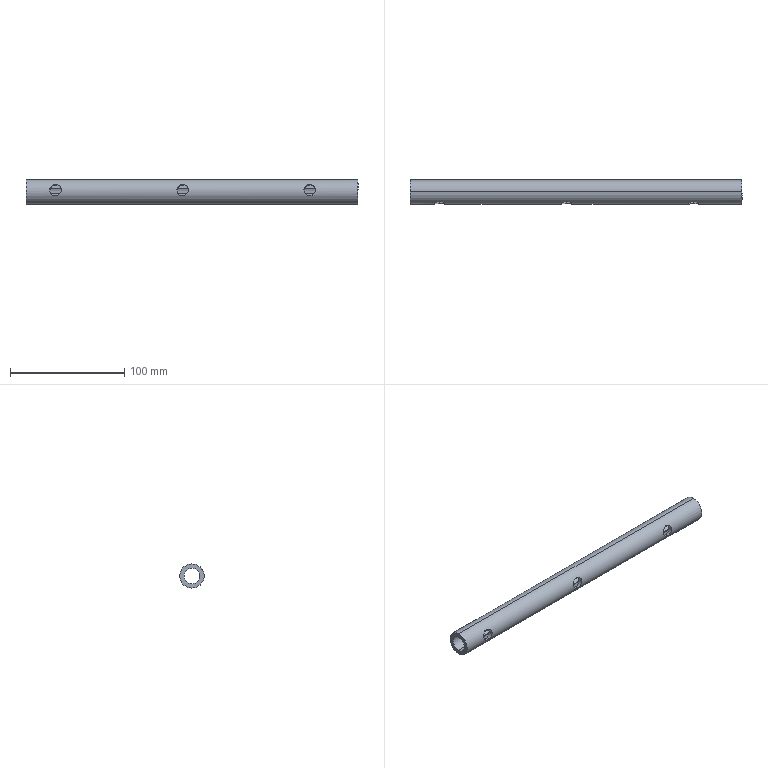Part | SolidWorks | features BaseBody 1 | 1 solid | 18 faces | box 290 x 21.234 x 21.234 mm | volume 58049 mm3 | cylinder 10 | plane 8 | commonest cylinder face diameters 10 x6 13.868 x2 21.234 x2
STEP:
#1=CARTESIAN_POINT('',(302.268,-63.762,6.934));
#2=VERTEX_POINT('',#1);
#3=CARTESIAN_POINT('',(302.268,-63.762,-6.934));
#4=VERTEX_POINT('',#3);
#5=CARTESIAN_POINT('',(302.268,-63.762,0.));
#6=DIRECTION('',(1.,0.,0.));
#7=DIRECTION('',(0.,0.,1.));
#8=AXIS2_PLACEMENT_3D('',#5,#6,#7);
#9=CIRCLE('',#8,6.934);
#10=EDGE_CURVE('',#2,#4,#9,.T.);
#11=ORIENTED_EDGE('',*,*,#10,.F.);
#12=CARTESIAN_POINT('',(302.268,-63.762,0.));
#13=DIRECTION('',(1.,0.,0.));
#14=DIRECTION('',(0.,0.,-1.));
#15=AXIS2_PLACEMENT_3D('',#12,#13,#14);
#16=CIRCLE('',#15,6.934);
#17=EDGE_CURVE('',#4,#2,#16,.T.);
#18=ORIENTED_EDGE('',*,*,#17,.F.);
#19=EDGE_LOOP('',(#11,#18));
#20=FACE_BOUND('',#19,.T.);
#21=CARTESIAN_POINT('',(302.268,-63.762,10.617));
#22=VERTEX_POINT('',#21);
#23=CARTESIAN_POINT('',(302.268,-63.762,-10.617));
#24=VERTEX_POINT('',#23);
#25=CARTESIAN_POINT('',(302.268,-63.762,0.));
#26=DIRECTION('',(-1.,0.,0.));
#27=DIRECTION('',(0.,0.,1.));
#28=AXIS2_PLACEMENT_3D('',#25,#26,#27);
#29=CIRCLE('',#28,10.617);
#30=EDGE_CURVE('',#22,#24,#29,.T.);
#31=ORIENTED_EDGE('',*,*,#30,.F.);
#32=CARTESIAN_POINT('',(302.268,-63.762,0.));
#33=DIRECTION('',(-1.,0.,0.));
#34=DIRECTION('',(0.,0.,-1.));
#35=AXIS2_PLACEMENT_3D('',#32,#33,#34);
#36=CIRCLE('',#35,10.617);
#37=EDGE_CURVE('',#24,#22,#36,.T.);
#38=ORIENTED_EDGE('',*,*,#37,.F.);
#39=EDGE_LOOP('',(#31,#38));
#40=FACE_OUTER_BOUND('',#39,.T.);
#41=CARTESIAN_POINT('',(302.268,-63.762,0.));
#42=DIRECTION('',(1.,0.,0.));
#43=DIRECTION('',(0.,1.,0.));
#44=AXIS2_PLACEMENT_3D('',#41,#42,#43);
#45=PLANE('',#44);
#46=ADVANCED_FACE('',(#20,#40),#45,.T.);
#47=CARTESIAN_POINT('',(12.268,-63.762,6.934));
#48=VERTEX_POINT('',#47);
#49=CARTESIAN_POINT('',(12.268,-63.762,-6.934));
#50=VERTEX_POINT('',#49);
#51=CARTESIAN_POINT('',(12.268,-63.762,0.));
#52=DIRECTION('',(-1.,0.,0.));
#53=DIRECTION('',(0.,0.,1.));
#54=AXIS2_PLACEMENT_3D('',#51,#52,#53);
#55=CIRCLE('',#54,6.934);
#56=EDGE_CURVE('',#48,#50,#55,.T.);
#57=ORIENTED_EDGE('',*,*,#56,.F.);
#58=CARTESIAN_POINT('',(12.268,-63.762,0.));
#59=DIRECTION('',(-1.,0.,0.));
#60=DIRECTION('',(0.,0.,-1.));
#61=AXIS2_PLACEMENT_3D('',#58,#59,#60);
#62=CIRCLE('',#61,6.934);
#63=EDGE_CURVE('',#50,#48,#62,.T.);
#64=ORIENTED_EDGE('',*,*,#63,.F.);
#65=EDGE_LOOP('',(#57,#64));
#66=FACE_BOUND('',#65,.T.);
#67=CARTESIAN_POINT('',(12.268,-63.762,10.617));
#68=VERTEX_POINT('',#67);
#69=CARTESIAN_POINT('',(12.268,-63.762,-10.617));
#70=VERTEX_POINT('',#69);
#71=CARTESIAN_POINT('',(12.268,-63.762,0.));
#72=DIRECTION('',(1.,0.,0.));
#73=DIRECTION('',(0.,0.,1.));
#74=AXIS2_PLACEMENT_3D('',#71,#72,#73);
#75=CIRCLE('',#74,10.617);
#76=EDGE_CURVE('',#68,#70,#75,.T.);
#77=ORIENTED_EDGE('',*,*,#76,.F.);
#78=CARTESIAN_POINT('',(12.268,-63.762,0.));
#79=DIRECTION('',(1.,0.,0.));
#80=DIRECTION('',(0.,0.,-1.));
#81=AXIS2_PLACEMENT_3D('',#78,#79,#80);
#82=CIRCLE('',#81,10.617);
#83=EDGE_CURVE('',#70,#68,#82,.T.);
#84=ORIENTED_EDGE('',*,*,#83,.F.);
#85=EDGE_LOOP('',(#77,#84));
#86=FACE_OUTER_BOUND('',#85,.T.);
#87=CARTESIAN_POINT('',(12.268,-63.762,0.));
#88=DIRECTION('',(-1.,0.,0.));
#89=DIRECTION('',(0.,0.,1.));
#90=AXIS2_PLACEMENT_3D('',#87,#88,#89);
#91=PLANE('',#90);
#92=ADVANCED_FACE('',(#66,#86),#91,.T.);
#93=ORIENTED_EDGE('',*,*,#83,.T.);
#94=CARTESIAN_POINT('',(302.268,-63.762,10.617));
#95=DIRECTION('',(-1.,0.,0.));
#96=VECTOR('',#95,1000.);
#97=LINE('',#94,#96);
#98=EDGE_CURVE('',#22,#68,#97,.T.);
#99=ORIENTED_EDGE('',*,*,#98,.F.);
#100=ORIENTED_EDGE('',*,*,#30,.T.);
#101=CARTESIAN_POINT('',(12.268,-63.762,-10.617));
#102=DIRECTION('',(1.,0.,0.));
#103=VECTOR('',#102,1000.);
#104=LINE('',#101,#103);
#105=EDGE_CURVE('',#70,#24,#104,.T.);
#106=ORIENTED_EDGE('',*,*,#105,.F.);
#107=EDGE_LOOP('',(#93,#99,#100,#106));
#108=FACE_OUTER_BOUND('',#107,.T.);
#109=CARTESIAN_POINT('',(302.268,-63.762,0.));
#110=DIRECTION('',(-1.,0.,0.));
#111=DIRECTION('',(0.,0.,1.));
#112=AXIS2_PLACEMENT_3D('',#109,#110,#111);
#113=CYLINDRICAL_SURFACE('',#112,10.617);
#114=ADVANCED_FACE('',(#108),#113,.T.);
#115=CARTESIAN_POINT('',(38.081,-72.117,6.55));
#116=VERTEX_POINT('',#115);
#117=CARTESIAN_POINT('',(33.081,-74.218,1.844));
#118=VERTEX_POINT('',#117);
#119=CARTESIAN_POINT('',(38.081,-72.117,6.55));
#120=CARTESIAN_POINT('',(37.773,-72.117,6.55));
#121=CARTESIAN_POINT('',(37.455,-72.138,6.525));
#122=CARTESIAN_POINT('',(36.97,-72.203,6.441));
#123=CARTESIAN_POINT('',(36.807,-72.23,6.406));
#124=CARTESIAN_POINT('',(36.562,-72.279,6.34));
#125=CARTESIAN_POINT('',(36.44,-72.305,6.304));
#126=CARTESIAN_POINT('',(36.297,-72.34,6.256));
#127=CARTESIAN_POINT('',(36.226,-72.358,6.231));
#128=CARTESIAN_POINT('',(36.191,-72.368,6.218));
#129=CARTESIAN_POINT('',(36.173,-72.372,6.211));
#130=CARTESIAN_POINT('',(36.165,-72.374,6.209));
#131=CARTESIAN_POINT('',(36.16,-72.376,6.207));
#132=CARTESIAN_POINT('',(36.157,-72.377,6.205));
#133=CARTESIAN_POINT('',(35.973,-72.427,6.136));
#134=CARTESIAN_POINT('',(35.735,-72.501,6.037));
#135=CARTESIAN_POINT('',(35.321,-72.655,5.805));
#136=CARTESIAN_POINT('',(35.173,-72.714,5.714));
#137=CARTESIAN_POINT('',(34.943,-72.814,5.551));
#138=CARTESIAN_POINT('',(34.865,-72.85,5.492));
#139=CARTESIAN_POINT('',(34.747,-72.906,5.397));
#140=CARTESIAN_POINT('',(34.688,-72.935,5.347));
#141=CARTESIAN_POINT('',(34.618,-72.97,5.286));
#142=CARTESIAN_POINT('',(34.588,-72.985,5.259));
#143=CARTESIAN_POINT('',(34.568,-72.995,5.241));
#144=CARTESIAN_POINT('',(34.557,-73.001,5.231));
#145=CARTESIAN_POINT('',(34.257,-73.157,4.955));
#146=CARTESIAN_POINT('',(34.033,-73.294,4.68));
#147=CARTESIAN_POINT('',(33.772,-73.471,4.293));
#148=CARTESIAN_POINT('',(33.697,-73.526,4.168));
#149=CARTESIAN_POINT('',(33.601,-73.6,3.99));
#150=CARTESIAN_POINT('',(33.571,-73.624,3.932));
#151=CARTESIAN_POINT('',(33.53,-73.657,3.848));
#152=CARTESIAN_POINT('',(33.51,-73.673,3.806));
#153=CARTESIAN_POINT('',(33.489,-73.691,3.759));
#154=CARTESIAN_POINT('',(33.478,-73.7,3.736));
#155=CARTESIAN_POINT('',(33.474,-73.704,3.726));
#156=CARTESIAN_POINT('',(33.471,-73.706,3.719));
#157=CARTESIAN_POINT('',(33.47,-73.707,3.718));
#158=CARTESIAN_POINT('',(33.201,-73.935,3.105));
#159=CARTESIAN_POINT('',(33.081,-74.108,2.463));
#160=CARTESIAN_POINT('',(33.081,-74.218,1.844));
#161=B_SPLINE_CURVE_WITH_KNOTS('',3,(#119,#120,#121,#122,#123,#124,#125,#126,#127,#128,#129,#130,#131,#132,#133,#134,#135,#136,#137,#138,#139,#140,#141,#142,#143,#144,#145,#146,#147,#148,#149,#150,#151,#152,#153,#154,#155,#156,#157,#158,#159,#160),.UNSPECIFIED.,.F.,.F.,(4,2,2,1,1,1,1,1,2,2,2,2,2,1,1,2,2,2,2,2,1,1,1,2,2,4),(0.,0.125,0.1875,0.2188,0.2344,0.2422,0.2461,0.248,0.249,0.25,0.375,0.4375,0.4688,0.4844,0.4922,0.4961,0.5,0.625,0.6875,0.7188,0.7344,0.7422,0.7461,0.748,0.75,1.),.UNSPECIFIED.);
#162=EDGE_CURVE('',#116,#118,#161,.T.);
#163=ORIENTED_EDGE('',*,*,#162,.F.);
#164=CARTESIAN_POINT('',(43.081,-74.218,1.844));
#165=VERTEX_POINT('',#164);
#166=CARTESIAN_POINT('',(43.081,-74.218,1.844));
#167=CARTESIAN_POINT('',(43.081,-74.163,2.153));
#168=CARTESIAN_POINT('',(43.051,-74.092,2.468));
#169=CARTESIAN_POINT('',(42.956,-73.965,2.939));
#170=CARTESIAN_POINT('',(42.916,-73.918,3.096));
#171=CARTESIAN_POINT('',(42.842,-73.844,3.329));
#172=CARTESIAN_POINT('',(42.802,-73.805,3.445));
#173=CARTESIAN_POINT('',(42.75,-73.757,3.579));
#174=CARTESIAN_POINT('',(42.722,-73.733,3.646));
#175=CARTESIAN_POINT('',(42.708,-73.721,3.68));
#176=CARTESIAN_POINT('',(42.702,-73.716,3.694));
#177=CARTESIAN_POINT('',(42.698,-73.712,3.703));
#178=CARTESIAN_POINT('',(42.695,-73.71,3.71));
#179=CARTESIAN_POINT('',(42.601,-73.63,3.923));
#180=CARTESIAN_POINT('',(42.477,-73.531,4.164));
#181=CARTESIAN_POINT('',(42.216,-73.353,4.551));
#182=CARTESIAN_POINT('',(42.116,-73.289,4.684));
#183=CARTESIAN_POINT('',(41.945,-73.187,4.885));
#184=CARTESIAN_POINT('',(41.884,-73.152,4.953));
#185=CARTESIAN_POINT('',(41.787,-73.098,5.054));
#186=CARTESIAN_POINT('',(41.737,-73.071,5.105));
#187=CARTESIAN_POINT('',(41.676,-73.038,5.164));
#188=CARTESIAN_POINT('',(41.65,-73.024,5.189));
#189=CARTESIAN_POINT('',(41.632,-73.015,5.206));
#190=CARTESIAN_POINT('',(41.624,-73.011,5.214));
#191=CARTESIAN_POINT('',(41.294,-72.839,5.517));
#192=CARTESIAN_POINT('',(40.979,-72.707,5.728));
#193=CARTESIAN_POINT('',(40.564,-72.552,5.96));
#194=CARTESIAN_POINT('',(40.436,-72.508,6.023));
#195=CARTESIAN_POINT('',(40.261,-72.452,6.102));
#196=CARTESIAN_POINT('',(40.205,-72.434,6.126));
#197=CARTESIAN_POINT('',(40.127,-72.411,6.158));
#198=CARTESIAN_POINT('',(40.089,-72.4,6.173));
#199=CARTESIAN_POINT('',(40.047,-72.388,6.189));
#200=CARTESIAN_POINT('',(40.026,-72.383,6.197));
#201=CARTESIAN_POINT('',(40.016,-72.38,6.201));
#202=CARTESIAN_POINT('',(40.012,-72.379,6.203));
#203=CARTESIAN_POINT('',(40.009,-72.378,6.204));
#204=CARTESIAN_POINT('',(40.009,-72.378,6.204));
#205=CARTESIAN_POINT('',(39.358,-72.202,6.449));
#206=CARTESIAN_POINT('',(38.696,-72.117,6.55));
#207=CARTESIAN_POINT('',(38.081,-72.117,6.55));
#208=B_SPLINE_CURVE_WITH_KNOTS('',3,(#166,#167,#168,#169,#170,#171,#172,#173,#174,#175,#176,#177,#178,#179,#180,#181,#182,#183,#184,#185,#186,#187,#188,#189,#190,#191,#192,#193,#194,#195,#196,#197,#198,#199,#200,#201,#202,#203,#204,#205,#206,#207),.UNSPECIFIED.,.F.,.F.,(4,2,2,1,1,1,1,2,2,2,2,2,1,1,2,2,2,2,2,1,1,1,1,2,2,4),(0.,0.125,0.1875,0.2187,0.2344,0.2422,0.2461,0.248,0.25,0.375,0.4375,0.4688,0.4844,0.4922,0.4961,0.5,0.625,0.6875,0.7187,0.7344,0.7422,0.7461,0.748,0.749,0.75,1.),.UNSPECIFIED.);
#209=EDGE_CURVE('',#165,#116,#208,.T.);
#210=ORIENTED_EDGE('',*,*,#209,.F.);
#211=CARTESIAN_POINT('',(38.081,-73.854,-3.298));
#212=VERTEX_POINT('',#211);
#213=CARTESIAN_POINT('',(38.081,-73.854,-3.298));
#214=CARTESIAN_POINT('',(38.388,-73.854,-3.298));
#215=CARTESIAN_POINT('',(38.707,-73.865,-3.267));
#216=CARTESIAN_POINT('',(39.192,-73.897,-3.166));
#217=CARTESIAN_POINT('',(39.355,-73.91,-3.123));
#218=CARTESIAN_POINT('',(39.599,-73.933,-3.044));
#219=CARTESIAN_POINT('',(39.722,-73.946,-3.002));
#220=CARTESIAN_POINT('',(39.864,-73.962,-2.945));
#221=CARTESIAN_POINT('',(39.935,-73.971,-2.915));
#222=CARTESIAN_POINT('',(39.971,-73.975,-2.9));
#223=CARTESIAN_POINT('',(39.989,-73.978,-2.892));
#224=CARTESIAN_POINT('',(39.996,-73.978,-2.888));
#225=CARTESIAN_POINT('',(40.001,-73.979,-2.886));
#226=CARTESIAN_POINT('',(40.005,-73.98,-2.884));
#227=CARTESIAN_POINT('',(40.189,-74.003,-2.803));
#228=CARTESIAN_POINT('',(40.426,-74.038,-2.684));
#229=CARTESIAN_POINT('',(40.841,-74.104,-2.413));
#230=CARTESIAN_POINT('',(40.988,-74.128,-2.307));
#231=CARTESIAN_POINT('',(41.218,-74.167,-2.12));
#232=CARTESIAN_POINT('',(41.296,-74.18,-2.052));
#233=CARTESIAN_POINT('',(41.415,-74.2,-1.944));
#234=CARTESIAN_POINT('',(41.474,-74.21,-1.887));
#235=CARTESIAN_POINT('',(41.544,-74.222,-1.818));
#236=CARTESIAN_POINT('',(41.574,-74.227,-1.788));
#237=CARTESIAN_POINT('',(41.594,-74.231,-1.767));
#238=CARTESIAN_POINT('',(41.605,-74.233,-1.756));
#239=CARTESIAN_POINT('',(41.904,-74.285,-1.443));
#240=CARTESIAN_POINT('',(42.128,-74.32,-1.137));
#241=CARTESIAN_POINT('',(42.39,-74.354,-0.7131));
#242=CARTESIAN_POINT('',(42.464,-74.363,-0.5772));
#243=CARTESIAN_POINT('',(42.561,-74.371,-0.3845));
#244=CARTESIAN_POINT('',(42.591,-74.374,-0.3221));
#245=CARTESIAN_POINT('',(42.632,-74.376,-0.2316));
#246=CARTESIAN_POINT('',(42.651,-74.377,-0.1871));
#247=CARTESIAN_POINT('',(42.673,-74.378,-0.1365));
#248=CARTESIAN_POINT('',(42.683,-74.378,-0.1116));
#249=CARTESIAN_POINT('',(42.688,-74.378,-0.101));
#250=CARTESIAN_POINT('',(42.691,-74.378,-0.09396));
#251=CARTESIAN_POINT('',(42.692,-74.379,-0.092));
#252=CARTESIAN_POINT('',(42.96,-74.384,0.5614));
#253=CARTESIAN_POINT('',(43.081,-74.327,1.224));
#254=CARTESIAN_POINT('',(43.081,-74.218,1.844));
#255=B_SPLINE_CURVE_WITH_KNOTS('',3,(#213,#214,#215,#216,#217,#218,#219,#220,#221,#222,#223,#224,#225,#226,#227,#228,#229,#230,#231,#232,#233,#234,#235,#236,#237,#238,#239,#240,#241,#242,#243,#244,#245,#246,#247,#248,#249,#250,#251,#252,#253,#254),.UNSPECIFIED.,.F.,.F.,(4,2,2,1,1,1,1,1,2,2,2,2,2,1,1,2,2,2,2,2,1,1,1,2,2,4),(0.,0.125,0.1875,0.2187,0.2344,0.2422,0.2461,0.248,0.249,0.25,0.375,0.4375,0.4687,0.4844,0.4922,0.4961,0.5,0.625,0.6875,0.7188,0.7344,0.7422,0.7461,0.748,0.75,1.),.UNSPECIFIED.);
#256=EDGE_CURVE('',#212,#165,#255,.T.);
#257=ORIENTED_EDGE('',*,*,#256,.F.);
#258=CARTESIAN_POINT('',(33.081,-74.218,1.844));
#259=CARTESIAN_POINT('',(33.081,-74.272,1.534));
#260=CARTESIAN_POINT('',(33.111,-74.314,1.214));
#261=CARTESIAN_POINT('',(33.206,-74.355,0.7275));
#262=CARTESIAN_POINT('',(33.246,-74.365,0.5645));
#263=CARTESIAN_POINT('',(33.319,-74.374,0.3198));
#264=CARTESIAN_POINT('',(33.359,-74.377,0.1975));
#265=CARTESIAN_POINT('',(33.412,-74.379,0.05512));
#266=CARTESIAN_POINT('',(33.439,-74.379,-0.01596));
#267=CARTESIAN_POINT('',(33.454,-74.379,-0.05146));
#268=CARTESIAN_POINT('',(33.46,-74.379,-0.06667));
#269=CARTESIAN_POINT('',(33.464,-74.379,-0.0768));
#270=CARTESIAN_POINT('',(33.467,-74.379,-0.08343));
#271=CARTESIAN_POINT('',(33.56,-74.377,-0.3113));
#272=CARTESIAN_POINT('',(33.685,-74.366,-0.5716));
#273=CARTESIAN_POINT('',(33.946,-74.331,-0.9957));
#274=CARTESIAN_POINT('',(34.046,-74.317,-1.143));
#275=CARTESIAN_POINT('',(34.217,-74.29,-1.367));
#276=CARTESIAN_POINT('',(34.277,-74.28,-1.443));
#277=CARTESIAN_POINT('',(34.374,-74.264,-1.556));
#278=CARTESIAN_POINT('',(34.424,-74.256,-1.613));
#279=CARTESIAN_POINT('',(34.485,-74.245,-1.68));
#280=CARTESIAN_POINT('',(34.512,-74.241,-1.708));
#281=CARTESIAN_POINT('',(34.53,-74.237,-1.727));
#282=CARTESIAN_POINT('',(34.538,-74.236,-1.736));
#283=CARTESIAN_POINT('',(34.867,-74.179,-2.08));
#284=CARTESIAN_POINT('',(35.183,-74.126,-2.323));
#285=CARTESIAN_POINT('',(35.597,-74.06,-2.594));
#286=CARTESIAN_POINT('',(35.726,-74.04,-2.668));
#287=CARTESIAN_POINT('',(35.901,-74.014,-2.762));
#288=CARTESIAN_POINT('',(35.956,-74.007,-2.79));
#289=CARTESIAN_POINT('',(36.035,-73.996,-2.828));
#290=CARTESIAN_POINT('',(36.073,-73.99,-2.846));
#291=CARTESIAN_POINT('',(36.115,-73.985,-2.866));
#292=CARTESIAN_POINT('',(36.135,-73.982,-2.875));
#293=CARTESIAN_POINT('',(36.145,-73.981,-2.879));
#294=CARTESIAN_POINT('',(36.15,-73.98,-2.881));
#295=CARTESIAN_POINT('',(36.152,-73.98,-2.883));
#296=CARTESIAN_POINT('',(36.153,-73.98,-2.883));
#297=CARTESIAN_POINT('',(36.804,-73.898,-3.173));
#298=CARTESIAN_POINT('',(37.466,-73.854,-3.298));
#299=CARTESIAN_POINT('',(38.081,-73.854,-3.298));
#300=B_SPLINE_CURVE_WITH_KNOTS('',3,(#258,#259,#260,#261,#262,#263,#264,#265,#266,#267,#268,#269,#270,#271,#272,#273,#274,#275,#276,#277,#278,#279,#280,#281,#282,#283,#284,#285,#286,#287,#288,#289,#290,#291,#292,#293,#294,#295,#296,#297,#298,#299),.UNSPECIFIED.,.F.,.F.,(4,2,2,1,1,1,1,2,2,2,2,2,1,1,2,2,2,2,2,1,1,1,1,2,2,4),(0.,0.125,0.1875,0.2188,0.2344,0.2422,0.2461,0.248,0.25,0.375,0.4375,0.4688,0.4844,0.4922,0.4961,0.5,0.625,0.6875,0.7188,0.7344,0.7422,0.7461,0.748,0.749,0.75,1.),.UNSPECIFIED.);
#301=EDGE_CURVE('',#118,#212,#300,.T.);
#302=ORIENTED_EDGE('',*,*,#301,.F.);
#303=EDGE_LOOP('',(#163,#210,#257,#302));
#304=FACE_BOUND('',#303,.T.);
#305=CARTESIAN_POINT('',(260.081,-72.117,6.55));
#306=VERTEX_POINT('',#305);
#307=CARTESIAN_POINT('',(255.081,-74.218,1.844));
#308=VERTEX_POINT('',#307);
#309=CARTESIAN_POINT('',(260.081,-72.117,6.55));
#310=CARTESIAN_POINT('',(259.773,-72.117,6.55));
#311=CARTESIAN_POINT('',(259.455,-72.138,6.525));
#312=CARTESIAN_POINT('',(258.97,-72.203,6.441));
#313=CARTESIAN_POINT('',(258.807,-72.23,6.406));
#314=CARTESIAN_POINT('',(258.562,-72.279,6.34));
#315=CARTESIAN_POINT('',(258.44,-72.305,6.304));
#316=CARTESIAN_POINT('',(258.297,-72.34,6.256));
#317=CARTESIAN_POINT('',(258.226,-72.358,6.231));
#318=CARTESIAN_POINT('',(258.191,-72.368,6.218));
#319=CARTESIAN_POINT('',(258.173,-72.372,6.211));
#320=CARTESIAN_POINT('',(258.165,-72.374,6.209));
#321=CARTESIAN_POINT('',(258.16,-72.376,6.207));
#322=CARTESIAN_POINT('',(258.157,-72.377,6.205));
#323=CARTESIAN_POINT('',(257.973,-72.427,6.136));
#324=CARTESIAN_POINT('',(257.735,-72.501,6.037));
#325=CARTESIAN_POINT('',(257.321,-72.655,5.805));
#326=CARTESIAN_POINT('',(257.173,-72.714,5.714));
#327=CARTESIAN_POINT('',(256.943,-72.814,5.551));
#328=CARTESIAN_POINT('',(256.865,-72.85,5.492));
#329=CARTESIAN_POINT('',(256.747,-72.906,5.397));
#330=CARTESIAN_POINT('',(256.688,-72.935,5.347));
#331=CARTESIAN_POINT('',(256.618,-72.97,5.286));
#332=CARTESIAN_POINT('',(256.588,-72.985,5.259));
#333=CARTESIAN_POINT('',(256.568,-72.995,5.241));
#334=CARTESIAN_POINT('',(256.557,-73.001,5.231));
#335=CARTESIAN_POINT('',(256.257,-73.157,4.955));
#336=CARTESIAN_POINT('',(256.033,-73.294,4.68));
#337=CARTESIAN_POINT('',(255.772,-73.471,4.293));
#338=CARTESIAN_POINT('',(255.697,-73.526,4.168));
#339=CARTESIAN_POINT('',(255.601,-73.6,3.99));
#340=CARTESIAN_POINT('',(255.571,-73.624,3.932));
#341=CARTESIAN_POINT('',(255.53,-73.657,3.848));
#342=CARTESIAN_POINT('',(255.51,-73.673,3.806));
#343=CARTESIAN_POINT('',(255.489,-73.691,3.759));
#344=CARTESIAN_POINT('',(255.478,-73.7,3.736));
#345=CARTESIAN_POINT('',(255.474,-73.704,3.726));
#346=CARTESIAN_POINT('',(255.471,-73.706,3.719));
#347=CARTESIAN_POINT('',(255.47,-73.707,3.718));
#348=CARTESIAN_POINT('',(255.201,-73.935,3.105));
#349=CARTESIAN_POINT('',(255.081,-74.108,2.463));
#350=CARTESIAN_POINT('',(255.081,-74.218,1.844));
#351=B_SPLINE_CURVE_WITH_KNOTS('',3,(#309,#310,#311,#312,#313,#314,#315,#316,#317,#318,#319,#320,#321,#322,#323,#324,#325,#326,#327,#328,#329,#330,#331,#332,#333,#334,#335,#336,#337,#338,#339,#340,#341,#342,#343,#344,#345,#346,#347,#348,#349,#350),.UNSPECIFIED.,.F.,.F.,(4,2,2,1,1,1,1,1,2,2,2,2,2,1,1,2,2,2,2,2,1,1,1,2,2,4),(0.,0.125,0.1875,0.2188,0.2344,0.2422,0.2461,0.248,0.249,0.25,0.375,0.4375,0.4688,0.4844,0.4922,0.4961,0.5,0.625,0.6875,0.7188,0.7344,0.7422,0.7461,0.748,0.75,1.),.UNSPECIFIED.);
#352=EDGE_CURVE('',#306,#308,#351,.T.);
#353=ORIENTED_EDGE('',*,*,#352,.F.);
#354=CARTESIAN_POINT('',(265.081,-74.218,1.844));
#355=VERTEX_POINT('',#354);
#356=CARTESIAN_POINT('',(265.081,-74.218,1.844));
#357=CARTESIAN_POINT('',(265.081,-74.163,2.153));
#358=CARTESIAN_POINT('',(265.051,-74.092,2.468));
#359=CARTESIAN_POINT('',(264.956,-73.965,2.939));
#360=CARTESIAN_POINT('',(264.916,-73.918,3.096));
#361=CARTESIAN_POINT('',(264.842,-73.844,3.329));
#362=CARTESIAN_POINT('',(264.802,-73.805,3.445));
#363=CARTESIAN_POINT('',(264.75,-73.757,3.579));
#364=CARTESIAN_POINT('',(264.722,-73.733,3.646));
#365=CARTESIAN_POINT('',(264.708,-73.721,3.68));
#366=CARTESIAN_POINT('',(264.702,-73.716,3.694));
#367=CARTESIAN_POINT('',(264.698,-73.712,3.703));
#368=CARTESIAN_POINT('',(264.695,-73.71,3.71));
#369=CARTESIAN_POINT('',(264.601,-73.63,3.923));
#370=CARTESIAN_POINT('',(264.477,-73.531,4.164));
#371=CARTESIAN_POINT('',(264.216,-73.353,4.551));
#372=CARTESIAN_POINT('',(264.116,-73.289,4.684));
#373=CARTESIAN_POINT('',(263.945,-73.187,4.885));
#374=CARTESIAN_POINT('',(263.884,-73.152,4.953));
#375=CARTESIAN_POINT('',(263.787,-73.098,5.054));
#376=CARTESIAN_POINT('',(263.737,-73.071,5.105));
#377=CARTESIAN_POINT('',(263.676,-73.038,5.164));
#378=CARTESIAN_POINT('',(263.65,-73.024,5.189));
#379=CARTESIAN_POINT('',(263.632,-73.015,5.206));
#380=CARTESIAN_POINT('',(263.624,-73.011,5.214));
#381=CARTESIAN_POINT('',(263.294,-72.839,5.517));
#382=CARTESIAN_POINT('',(262.979,-72.707,5.728));
#383=CARTESIAN_POINT('',(262.564,-72.552,5.96));
#384=CARTESIAN_POINT('',(262.436,-72.508,6.023));
#385=CARTESIAN_POINT('',(262.261,-72.452,6.102));
#386=CARTESIAN_POINT('',(262.205,-72.434,6.126));
#387=CARTESIAN_POINT('',(262.127,-72.411,6.158));
#388=CARTESIAN_POINT('',(262.089,-72.4,6.173));
#389=CARTESIAN_POINT('',(262.047,-72.388,6.189));
#390=CARTESIAN_POINT('',(262.026,-72.383,6.197));
#391=CARTESIAN_POINT('',(262.016,-72.38,6.201));
#392=CARTESIAN_POINT('',(262.012,-72.379,6.203));
#393=CARTESIAN_POINT('',(262.009,-72.378,6.204));
#394=CARTESIAN_POINT('',(262.009,-72.378,6.204));
#395=CARTESIAN_POINT('',(261.358,-72.202,6.449));
#396=CARTESIAN_POINT('',(260.696,-72.117,6.55));
#397=CARTESIAN_POINT('',(260.081,-72.117,6.55));
#398=B_SPLINE_CURVE_WITH_KNOTS('',3,(#356,#357,#358,#359,#360,#361,#362,#363,#364,#365,#366,#367,#368,#369,#370,#371,#372,#373,#374,#375,#376,#377,#378,#379,#380,#381,#382,#383,#384,#385,#386,#387,#388,#389,#390,#391,#392,#393,#394,#395,#396,#397),.UNSPECIFIED.,.F.,.F.,(4,2,2,1,1,1,1,2,2,2,2,2,1,1,2,2,2,2,2,1,1,1,1,2,2,4),(0.,0.125,0.1875,0.2187,0.2344,0.2422,0.2461,0.248,0.25,0.375,0.4375,0.4688,0.4844,0.4922,0.4961,0.5,0.625,0.6875,0.7188,0.7344,0.7422,0.7461,0.748,0.749,0.75,1.),.UNSPECIFIED.);
#399=EDGE_CURVE('',#355,#306,#398,.T.);
#400=ORIENTED_EDGE('',*,*,#399,.F.);
#401=CARTESIAN_POINT('',(260.081,-73.854,-3.298));
#402=VERTEX_POINT('',#401);
#403=CARTESIAN_POINT('',(260.081,-73.854,-3.298));
#404=CARTESIAN_POINT('',(260.388,-73.854,-3.298));
#405=CARTESIAN_POINT('',(260.707,-73.865,-3.267));
#406=CARTESIAN_POINT('',(261.192,-73.897,-3.166));
#407=CARTESIAN_POINT('',(261.355,-73.91,-3.123));
#408=CARTESIAN_POINT('',(261.599,-73.933,-3.044));
#409=CARTESIAN_POINT('',(261.722,-73.946,-3.002));
#410=CARTESIAN_POINT('',(261.864,-73.962,-2.945));
#411=CARTESIAN_POINT('',(261.935,-73.971,-2.915));
#412=CARTESIAN_POINT('',(261.971,-73.975,-2.9));
#413=CARTESIAN_POINT('',(261.989,-73.978,-2.892));
#414=CARTESIAN_POINT('',(261.996,-73.978,-2.888));
#415=CARTESIAN_POINT('',(262.001,-73.979,-2.886));
#416=CARTESIAN_POINT('',(262.005,-73.98,-2.884));
#417=CARTESIAN_POINT('',(262.189,-74.003,-2.803));
#418=CARTESIAN_POINT('',(262.426,-74.038,-2.684));
#419=CARTESIAN_POINT('',(262.841,-74.104,-2.413));
#420=CARTESIAN_POINT('',(262.988,-74.128,-2.307));
#421=CARTESIAN_POINT('',(263.218,-74.167,-2.12));
#422=CARTESIAN_POINT('',(263.296,-74.18,-2.052));
#423=CARTESIAN_POINT('',(263.415,-74.2,-1.944));
#424=CARTESIAN_POINT('',(263.474,-74.21,-1.887));
#425=CARTESIAN_POINT('',(263.544,-74.222,-1.818));
#426=CARTESIAN_POINT('',(263.574,-74.227,-1.788));
#427=CARTESIAN_POINT('',(263.594,-74.231,-1.767));
#428=CARTESIAN_POINT('',(263.605,-74.233,-1.756));
#429=CARTESIAN_POINT('',(263.904,-74.285,-1.443));
#430=CARTESIAN_POINT('',(264.128,-74.32,-1.137));
#431=CARTESIAN_POINT('',(264.39,-74.354,-0.7131));
#432=CARTESIAN_POINT('',(264.464,-74.363,-0.5772));
#433=CARTESIAN_POINT('',(264.561,-74.371,-0.3845));
#434=CARTESIAN_POINT('',(264.591,-74.374,-0.3221));
#435=CARTESIAN_POINT('',(264.632,-74.376,-0.2316));
#436=CARTESIAN_POINT('',(264.651,-74.377,-0.1871));
#437=CARTESIAN_POINT('',(264.673,-74.378,-0.1365));
#438=CARTESIAN_POINT('',(264.683,-74.378,-0.1116));
#439=CARTESIAN_POINT('',(264.688,-74.378,-0.101));
#440=CARTESIAN_POINT('',(264.691,-74.378,-0.09396));
#441=CARTESIAN_POINT('',(264.692,-74.379,-0.092));
#442=CARTESIAN_POINT('',(264.96,-74.384,0.5614));
#443=CARTESIAN_POINT('',(265.081,-74.327,1.224));
#444=CARTESIAN_POINT('',(265.081,-74.218,1.844));
#445=B_SPLINE_CURVE_WITH_KNOTS('',3,(#403,#404,#405,#406,#407,#408,#409,#410,#411,#412,#413,#414,#415,#416,#417,#418,#419,#420,#421,#422,#423,#424,#425,#426,#427,#428,#429,#430,#431,#432,#433,#434,#435,#436,#437,#438,#439,#440,#441,#442,#443,#444),.UNSPECIFIED.,.F.,.F.,(4,2,2,1,1,1,1,1,2,2,2,2,2,1,1,2,2,2,2,2,1,1,1,2,2,4),(0.,0.125,0.1875,0.2187,0.2344,0.2422,0.2461,0.248,0.249,0.25,0.375,0.4375,0.4687,0.4844,0.4922,0.4961,0.5,0.625,0.6875,0.7187,0.7344,0.7422,0.7461,0.748,0.75,1.),.UNSPECIFIED.);
#446=EDGE_CURVE('',#402,#355,#445,.T.);
#447=ORIENTED_EDGE('',*,*,#446,.F.);
#448=CARTESIAN_POINT('',(255.081,-74.218,1.844));
#449=CARTESIAN_POINT('',(255.081,-74.272,1.534));
#450=CARTESIAN_POINT('',(255.111,-74.314,1.214));
#451=CARTESIAN_POINT('',(255.206,-74.355,0.7275));
#452=CARTESIAN_POINT('',(255.246,-74.365,0.5645));
#453=CARTESIAN_POINT('',(255.319,-74.374,0.3198));
#454=CARTESIAN_POINT('',(255.359,-74.377,0.1975));
#455=CARTESIAN_POINT('',(255.412,-74.379,0.05512));
#456=CARTESIAN_POINT('',(255.439,-74.379,-0.01596));
#457=CARTESIAN_POINT('',(255.454,-74.379,-0.05146));
#458=CARTESIAN_POINT('',(255.46,-74.379,-0.06667));
#459=CARTESIAN_POINT('',(255.464,-74.379,-0.0768));
#460=CARTESIAN_POINT('',(255.467,-74.379,-0.08343));
#461=CARTESIAN_POINT('',(255.56,-74.377,-0.3113));
#462=CARTESIAN_POINT('',(255.685,-74.366,-0.5716));
#463=CARTESIAN_POINT('',(255.946,-74.331,-0.9957));
#464=CARTESIAN_POINT('',(256.046,-74.317,-1.143));
#465=CARTESIAN_POINT('',(256.217,-74.29,-1.367));
#466=CARTESIAN_POINT('',(256.277,-74.28,-1.443));
#467=CARTESIAN_POINT('',(256.374,-74.264,-1.556));
#468=CARTESIAN_POINT('',(256.424,-74.256,-1.613));
#469=CARTESIAN_POINT('',(256.485,-74.245,-1.68));
#470=CARTESIAN_POINT('',(256.512,-74.241,-1.708));
#471=CARTESIAN_POINT('',(256.53,-74.237,-1.727));
#472=CARTESIAN_POINT('',(256.538,-74.236,-1.736));
#473=CARTESIAN_POINT('',(256.867,-74.179,-2.08));
#474=CARTESIAN_POINT('',(257.183,-74.126,-2.323));
#475=CARTESIAN_POINT('',(257.597,-74.06,-2.594));
#476=CARTESIAN_POINT('',(257.726,-74.04,-2.668));
#477=CARTESIAN_POINT('',(257.901,-74.014,-2.762));
#478=CARTESIAN_POINT('',(257.956,-74.007,-2.79));
#479=CARTESIAN_POINT('',(258.035,-73.996,-2.828));
#480=CARTESIAN_POINT('',(258.073,-73.99,-2.846));
#481=CARTESIAN_POINT('',(258.115,-73.985,-2.866));
#482=CARTESIAN_POINT('',(258.135,-73.982,-2.875));
#483=CARTESIAN_POINT('',(258.145,-73.981,-2.879));
#484=CARTESIAN_POINT('',(258.15,-73.98,-2.881));
#485=CARTESIAN_POINT('',(258.152,-73.98,-2.883));
#486=CARTESIAN_POINT('',(258.153,-73.98,-2.883));
#487=CARTESIAN_POINT('',(258.804,-73.898,-3.173));
#488=CARTESIAN_POINT('',(259.466,-73.854,-3.298));
#489=CARTESIAN_POINT('',(260.081,-73.854,-3.298));
#490=B_SPLINE_CURVE_WITH_KNOTS('',3,(#448,#449,#450,#451,#452,#453,#454,#455,#456,#457,#458,#459,#460,#461,#462,#463,#464,#465,#466,#467,#468,#469,#470,#471,#472,#473,#474,#475,#476,#477,#478,#479,#480,#481,#482,#483,#484,#485,#486,#487,#488,#489),.UNSPECIFIED.,.F.,.F.,(4,2,2,1,1,1,1,2,2,2,2,2,1,1,2,2,2,2,2,1,1,1,1,2,2,4),(0.,0.125,0.1875,0.2187,0.2344,0.2422,0.2461,0.248,0.25,0.375,0.4375,0.4687,0.4844,0.4922,0.4961,0.5,0.625,0.6875,0.7187,0.7344,0.7422,0.7461,0.748,0.749,0.75,1.),.UNSPECIFIED.);
#491=EDGE_CURVE('',#308,#402,#490,.T.);
#492=ORIENTED_EDGE('',*,*,#491,.F.);
#493=EDGE_LOOP('',(#353,#400,#447,#492));
#494=FACE_BOUND('',#493,.T.);
#495=CARTESIAN_POINT('',(149.081,-72.117,6.55));
#496=VERTEX_POINT('',#495);
#497=CARTESIAN_POINT('',(144.081,-74.218,1.844));
#498=VERTEX_POINT('',#497);
#499=CARTESIAN_POINT('',(149.081,-72.117,6.55));
#500=CARTESIAN_POINT('',(148.773,-72.117,6.55));
#501=CARTESIAN_POINT('',(148.455,-72.138,6.525));
#502=CARTESIAN_POINT('',(147.97,-72.203,6.441));
#503=CARTESIAN_POINT('',(147.807,-72.23,6.406));
#504=CARTESIAN_POINT('',(147.562,-72.279,6.34));
#505=CARTESIAN_POINT('',(147.44,-72.305,6.304));
#506=CARTESIAN_POINT('',(147.297,-72.34,6.256));
#507=CARTESIAN_POINT('',(147.226,-72.358,6.231));
#508=CARTESIAN_POINT('',(147.191,-72.368,6.218));
#509=CARTESIAN_POINT('',(147.173,-72.372,6.211));
#510=CARTESIAN_POINT('',(147.165,-72.374,6.209));
#511=CARTESIAN_POINT('',(147.16,-72.376,6.207));
#512=CARTESIAN_POINT('',(147.157,-72.377,6.205));
#513=CARTESIAN_POINT('',(146.973,-72.427,6.136));
#514=CARTESIAN_POINT('',(146.735,-72.501,6.037));
#515=CARTESIAN_POINT('',(146.321,-72.655,5.805));
#516=CARTESIAN_POINT('',(146.173,-72.714,5.714));
#517=CARTESIAN_POINT('',(145.943,-72.814,5.551));
#518=CARTESIAN_POINT('',(145.865,-72.85,5.492));
#519=CARTESIAN_POINT('',(145.747,-72.906,5.397));
#520=CARTESIAN_POINT('',(145.688,-72.935,5.347));
#521=CARTESIAN_POINT('',(145.618,-72.97,5.286));
#522=CARTESIAN_POINT('',(145.588,-72.985,5.259));
#523=CARTESIAN_POINT('',(145.568,-72.995,5.241));
#524=CARTESIAN_POINT('',(145.557,-73.001,5.231));
#525=CARTESIAN_POINT('',(145.257,-73.157,4.955));
#526=CARTESIAN_POINT('',(145.033,-73.294,4.68));
#527=CARTESIAN_POINT('',(144.772,-73.471,4.293));
#528=CARTESIAN_POINT('',(144.697,-73.526,4.168));
#529=CARTESIAN_POINT('',(144.601,-73.6,3.99));
#530=CARTESIAN_POINT('',(144.571,-73.624,3.932));
#531=CARTESIAN_POINT('',(144.53,-73.657,3.848));
#532=CARTESIAN_POINT('',(144.51,-73.673,3.806));
#533=CARTESIAN_POINT('',(144.489,-73.691,3.759));
#534=CARTESIAN_POINT('',(144.478,-73.7,3.736));
#535=CARTESIAN_POINT('',(144.474,-73.704,3.726));
#536=CARTESIAN_POINT('',(144.471,-73.706,3.719));
#537=CARTESIAN_POINT('',(144.47,-73.707,3.718));
#538=CARTESIAN_POINT('',(144.201,-73.935,3.105));
#539=CARTESIAN_POINT('',(144.081,-74.108,2.463));
#540=CARTESIAN_POINT('',(144.081,-74.218,1.844));
#541=B_SPLINE_CURVE_WITH_KNOTS('',3,(#499,#500,#501,#502,#503,#504,#505,#506,#507,#508,#509,#510,#511,#512,#513,#514,#515,#516,#517,#518,#519,#520,#521,#522,#523,#524,#525,#526,#527,#528,#529,#530,#531,#532,#533,#534,#535,#536,#537,#538,#539,#540),.UNSPECIFIED.,.F.,.F.,(4,2,2,1,1,1,1,1,2,2,2,2,2,1,1,2,2,2,2,2,1,1,1,2,2,4),(0.,0.125,0.1875,0.2187,0.2344,0.2422,0.2461,0.248,0.249,0.25,0.375,0.4375,0.4687,0.4844,0.4922,0.4961,0.5,0.625,0.6875,0.7187,0.7344,0.7422,0.7461,0.748,0.75,1.),.UNSPECIFIED.);
#542=EDGE_CURVE('',#496,#498,#541,.T.);
#543=ORIENTED_EDGE('',*,*,#542,.F.);
#544=CARTESIAN_POINT('',(154.081,-74.218,1.844));
#545=VERTEX_POINT('',#544);
#546=CARTESIAN_POINT('',(154.081,-74.218,1.844));
#547=CARTESIAN_POINT('',(154.081,-74.163,2.153));
#548=CARTESIAN_POINT('',(154.051,-74.092,2.468));
#549=CARTESIAN_POINT('',(153.956,-73.965,2.939));
#550=CARTESIAN_POINT('',(153.916,-73.918,3.096));
#551=CARTESIAN_POINT('',(153.842,-73.844,3.329));
#552=CARTESIAN_POINT('',(153.802,-73.805,3.445));
#553=CARTESIAN_POINT('',(153.75,-73.757,3.579));
#554=CARTESIAN_POINT('',(153.722,-73.733,3.646));
#555=CARTESIAN_POINT('',(153.708,-73.721,3.68));
#556=CARTESIAN_POINT('',(153.702,-73.716,3.694));
#557=CARTESIAN_POINT('',(153.698,-73.712,3.703));
#558=CARTESIAN_POINT('',(153.695,-73.71,3.71));
#559=CARTESIAN_POINT('',(153.601,-73.63,3.923));
#560=CARTESIAN_POINT('',(153.477,-73.531,4.164));
#561=CARTESIAN_POINT('',(153.216,-73.353,4.551));
#562=CARTESIAN_POINT('',(153.116,-73.289,4.684));
#563=CARTESIAN_POINT('',(152.945,-73.187,4.885));
#564=CARTESIAN_POINT('',(152.884,-73.152,4.953));
#565=CARTESIAN_POINT('',(152.787,-73.098,5.054));
#566=CARTESIAN_POINT('',(152.737,-73.071,5.105));
#567=CARTESIAN_POINT('',(152.676,-73.038,5.164));
#568=CARTESIAN_POINT('',(152.65,-73.024,5.189));
#569=CARTESIAN_POINT('',(152.632,-73.015,5.206));
#570=CARTESIAN_POINT('',(152.624,-73.011,5.214));
#571=CARTESIAN_POINT('',(152.294,-72.839,5.517));
#572=CARTESIAN_POINT('',(151.979,-72.707,5.728));
#573=CARTESIAN_POINT('',(151.564,-72.552,5.96));
#574=CARTESIAN_POINT('',(151.436,-72.508,6.023));
#575=CARTESIAN_POINT('',(151.261,-72.452,6.102));
#576=CARTESIAN_POINT('',(151.205,-72.434,6.126));
#577=CARTESIAN_POINT('',(151.127,-72.411,6.158));
#578=CARTESIAN_POINT('',(151.089,-72.4,6.173));
#579=CARTESIAN_POINT('',(151.047,-72.388,6.189));
#580=CARTESIAN_POINT('',(151.026,-72.383,6.197));
#581=CARTESIAN_POINT('',(151.016,-72.38,6.201));
#582=CARTESIAN_POINT('',(151.012,-72.379,6.203));
#583=CARTESIAN_POINT('',(151.009,-72.378,6.204));
#584=CARTESIAN_POINT('',(151.009,-72.378,6.204));
#585=CARTESIAN_POINT('',(150.358,-72.202,6.449));
#586=CARTESIAN_POINT('',(149.696,-72.117,6.55));
#587=CARTESIAN_POINT('',(149.081,-72.117,6.55));
#588=B_SPLINE_CURVE_WITH_KNOTS('',3,(#546,#547,#548,#549,#550,#551,#552,#553,#554,#555,#556,#557,#558,#559,#560,#561,#562,#563,#564,#565,#566,#567,#568,#569,#570,#571,#572,#573,#574,#575,#576,#577,#578,#579,#580,#581,#582,#583,#584,#585,#586,#587),.UNSPECIFIED.,.F.,.F.,(4,2,2,1,1,1,1,2,2,2,2,2,1,1,2,2,2,2,2,1,1,1,1,2,2,4),(0.,0.125,0.1875,0.2187,0.2344,0.2422,0.2461,0.248,0.25,0.375,0.4375,0.4687,0.4844,0.4922,0.4961,0.5,0.625,0.6875,0.7187,0.7344,0.7422,0.7461,0.748,0.749,0.75,1.),.UNSPECIFIED.);
#589=EDGE_CURVE('',#545,#496,#588,.T.);
#590=ORIENTED_EDGE('',*,*,#589,.F.);
#591=CARTESIAN_POINT('',(149.081,-73.854,-3.298));
#592=VERTEX_POINT('',#591);
#593=CARTESIAN_POINT('',(149.081,-73.854,-3.298));
#594=CARTESIAN_POINT('',(149.388,-73.854,-3.298));
#595=CARTESIAN_POINT('',(149.707,-73.865,-3.267));
#596=CARTESIAN_POINT('',(150.192,-73.897,-3.166));
#597=CARTESIAN_POINT('',(150.355,-73.91,-3.123));
#598=CARTESIAN_POINT('',(150.599,-73.933,-3.044));
#599=CARTESIAN_POINT('',(150.722,-73.946,-3.002));
#600=CARTESIAN_POINT('',(150.864,-73.962,-2.945));
#601=CARTESIAN_POINT('',(150.935,-73.971,-2.915));
#602=CARTESIAN_POINT('',(150.971,-73.975,-2.9));
#603=CARTESIAN_POINT('',(150.989,-73.978,-2.892));
#604=CARTESIAN_POINT('',(150.996,-73.978,-2.888));
#605=CARTESIAN_POINT('',(151.001,-73.979,-2.886));
#606=CARTESIAN_POINT('',(151.005,-73.98,-2.884));
#607=CARTESIAN_POINT('',(151.189,-74.003,-2.803));
#608=CARTESIAN_POINT('',(151.426,-74.038,-2.684));
#609=CARTESIAN_POINT('',(151.841,-74.104,-2.413));
#610=CARTESIAN_POINT('',(151.988,-74.128,-2.307));
#611=CARTESIAN_POINT('',(152.218,-74.167,-2.12));
#612=CARTESIAN_POINT('',(152.296,-74.18,-2.052));
#613=CARTESIAN_POINT('',(152.415,-74.2,-1.944));
#614=CARTESIAN_POINT('',(152.474,-74.21,-1.887));
#615=CARTESIAN_POINT('',(152.544,-74.222,-1.818));
#616=CARTESIAN_POINT('',(152.574,-74.227,-1.788));
#617=CARTESIAN_POINT('',(152.594,-74.231,-1.767));
#618=CARTESIAN_POINT('',(152.605,-74.233,-1.756));
#619=CARTESIAN_POINT('',(152.904,-74.285,-1.443));
#620=CARTESIAN_POINT('',(153.128,-74.32,-1.137));
#621=CARTESIAN_POINT('',(153.39,-74.354,-0.7131));
#622=CARTESIAN_POINT('',(153.464,-74.363,-0.5772));
#623=CARTESIAN_POINT('',(153.561,-74.371,-0.3845));
#624=CARTESIAN_POINT('',(153.591,-74.374,-0.3221));
#625=CARTESIAN_POINT('',(153.632,-74.376,-0.2316));
#626=CARTESIAN_POINT('',(153.651,-74.377,-0.1871));
#627=CARTESIAN_POINT('',(153.673,-74.378,-0.1365));
#628=CARTESIAN_POINT('',(153.683,-74.378,-0.1116));
#629=CARTESIAN_POINT('',(153.688,-74.378,-0.101));
#630=CARTESIAN_POINT('',(153.691,-74.378,-0.09396));
#631=CARTESIAN_POINT('',(153.692,-74.379,-0.092));
#632=CARTESIAN_POINT('',(153.96,-74.384,0.5614));
#633=CARTESIAN_POINT('',(154.081,-74.327,1.224));
#634=CARTESIAN_POINT('',(154.081,-74.218,1.844));
#635=B_SPLINE_CURVE_WITH_KNOTS('',3,(#593,#594,#595,#596,#597,#598,#599,#600,#601,#602,#603,#604,#605,#606,#607,#608,#609,#610,#611,#612,#613,#614,#615,#616,#617,#618,#619,#620,#621,#622,#623,#624,#625,#626,#627,#628,#629,#630,#631,#632,#633,#634),.UNSPECIFIED.,.F.,.F.,(4,2,2,1,1,1,1,1,2,2,2,2,2,1,1,2,2,2,2,2,1,1,1,2,2,4),(0.,0.125,0.1875,0.2188,0.2344,0.2422,0.2461,0.248,0.249,0.25,0.375,0.4375,0.4688,0.4844,0.4922,0.4961,0.5,0.625,0.6875,0.7187,0.7344,0.7422,0.7461,0.748,0.75,1.),.UNSPECIFIED.);
#636=EDGE_CURVE('',#592,#545,#635,.T.);
#637=ORIENTED_EDGE('',*,*,#636,.F.);
#638=CARTESIAN_POINT('',(144.081,-74.218,1.844));
#639=CARTESIAN_POINT('',(144.081,-74.272,1.534));
#640=CARTESIAN_POINT('',(144.111,-74.314,1.214));
#641=CARTESIAN_POINT('',(144.206,-74.355,0.7275));
#642=CARTESIAN_POINT('',(144.246,-74.365,0.5645));
#643=CARTESIAN_POINT('',(144.319,-74.374,0.3198));
#644=CARTESIAN_POINT('',(144.359,-74.377,0.1975));
#645=CARTESIAN_POINT('',(144.412,-74.379,0.05512));
#646=CARTESIAN_POINT('',(144.439,-74.379,-0.01596));
#647=CARTESIAN_POINT('',(144.454,-74.379,-0.05146));
#648=CARTESIAN_POINT('',(144.46,-74.379,-0.06667));
#649=CARTESIAN_POINT('',(144.464,-74.379,-0.0768));
#650=CARTESIAN_POINT('',(144.467,-74.379,-0.08343));
#651=CARTESIAN_POINT('',(144.56,-74.377,-0.3113));
#652=CARTESIAN_POINT('',(144.685,-74.366,-0.5716));
#653=CARTESIAN_POINT('',(144.946,-74.331,-0.9957));
#654=CARTESIAN_POINT('',(145.046,-74.317,-1.143));
#655=CARTESIAN_POINT('',(145.217,-74.29,-1.367));
#656=CARTESIAN_POINT('',(145.277,-74.28,-1.443));
#657=CARTESIAN_POINT('',(145.374,-74.264,-1.556));
#658=CARTESIAN_POINT('',(145.424,-74.256,-1.613));
#659=CARTESIAN_POINT('',(145.485,-74.245,-1.68));
#660=CARTESIAN_POINT('',(145.512,-74.241,-1.708));
#661=CARTESIAN_POINT('',(145.53,-74.237,-1.727));
#662=CARTESIAN_POINT('',(145.538,-74.236,-1.736));
#663=CARTESIAN_POINT('',(145.867,-74.179,-2.08));
#664=CARTESIAN_POINT('',(146.183,-74.126,-2.323));
#665=CARTESIAN_POINT('',(146.597,-74.06,-2.594));
#666=CARTESIAN_POINT('',(146.726,-74.04,-2.668));
#667=CARTESIAN_POINT('',(146.901,-74.014,-2.762));
#668=CARTESIAN_POINT('',(146.956,-74.007,-2.79));
#669=CARTESIAN_POINT('',(147.035,-73.996,-2.828));
#670=CARTESIAN_POINT('',(147.073,-73.99,-2.846));
#671=CARTESIAN_POINT('',(147.115,-73.985,-2.866));
#672=CARTESIAN_POINT('',(147.135,-73.982,-2.875));
#673=CARTESIAN_POINT('',(147.145,-73.981,-2.879));
#674=CARTESIAN_POINT('',(147.15,-73.98,-2.881));
#675=CARTESIAN_POINT('',(147.152,-73.98,-2.883));
#676=CARTESIAN_POINT('',(147.153,-73.98,-2.883));
#677=CARTESIAN_POINT('',(147.804,-73.898,-3.173));
#678=CARTESIAN_POINT('',(148.466,-73.854,-3.298));
#679=CARTESIAN_POINT('',(149.081,-73.854,-3.298));
#680=B_SPLINE_CURVE_WITH_KNOTS('',3,(#638,#639,#640,#641,#642,#643,#644,#645,#646,#647,#648,#649,#650,#651,#652,#653,#654,#655,#656,#657,#658,#659,#660,#661,#662,#663,#664,#665,#666,#667,#668,#669,#670,#671,#672,#673,#674,#675,#676,#677,#678,#679),.UNSPECIFIED.,.F.,.F.,(4,2,2,1,1,1,1,2,2,2,2,2,1,1,2,2,2,2,2,1,1,1,1,2,2,4),(0.,0.125,0.1875,0.2187,0.2344,0.2422,0.2461,0.248,0.25,0.375,0.4375,0.4687,0.4844,0.4922,0.4961,0.5,0.625,0.6875,0.7187,0.7344,0.7422,0.7461,0.748,0.749,0.75,1.),.UNSPECIFIED.);
#681=EDGE_CURVE('',#498,#592,#680,.T.);
#682=ORIENTED_EDGE('',*,*,#681,.F.);
#683=EDGE_LOOP('',(#543,#590,#637,#682));
#684=FACE_BOUND('',#683,.T.);
#685=ORIENTED_EDGE('',*,*,#105,.T.);
#686=ORIENTED_EDGE('',*,*,#37,.T.);
#687=ORIENTED_EDGE('',*,*,#98,.T.);
#688=ORIENTED_EDGE('',*,*,#76,.T.);
#689=EDGE_LOOP('',(#685,#686,#687,#688));
#690=FACE_OUTER_BOUND('',#689,.T.);
#691=CARTESIAN_POINT('',(302.268,-63.762,0.));
#692=DIRECTION('',(-1.,0.,0.));
#693=DIRECTION('',(0.,0.,1.));
#694=AXIS2_PLACEMENT_3D('',#691,#692,#693);
#695=CYLINDRICAL_SURFACE('',#694,10.617);
#696=ADVANCED_FACE('',(#304,#494,#684,#690),#695,.T.);
#697=CARTESIAN_POINT('',(42.631,-69.918,3.19));
#698=VERTEX_POINT('',#697);
#699=CARTESIAN_POINT('',(42.631,-70.638,-0.8921));
#700=VERTEX_POINT('',#699);
#701=CARTESIAN_POINT('',(42.631,-69.918,3.19));
#702=CARTESIAN_POINT('',(42.938,-70.244,2.563));
#703=CARTESIAN_POINT('',(43.081,-70.472,1.877));
#704=CARTESIAN_POINT('',(43.081,-70.709,0.5312));
#705=CARTESIAN_POINT('',(42.938,-70.729,-0.1908));
#706=CARTESIAN_POINT('',(42.631,-70.638,-0.8921));
#707=B_SPLINE_CURVE_WITH_KNOTS('',3,(#701,#702,#703,#704,#705,#706),.UNSPECIFIED.,.F.,.F.,(4,2,4),(0.,0.5,1.),.UNSPECIFIED.);
#708=EDGE_CURVE('',#698,#700,#707,.T.);
#709=ORIENTED_EDGE('',*,*,#708,.F.);
#710=CARTESIAN_POINT('',(33.531,-69.918,3.19));
#711=VERTEX_POINT('',#710);
#712=CARTESIAN_POINT('',(33.531,-69.918,3.19));
#713=DIRECTION('',(1.,0.,0.));
#714=VECTOR('',#713,1000.);
#715=LINE('',#712,#714);
#716=EDGE_CURVE('',#711,#698,#715,.T.);
#717=ORIENTED_EDGE('',*,*,#716,.F.);
#718=CARTESIAN_POINT('',(33.531,-70.638,-0.8921));
#719=VERTEX_POINT('',#718);
#720=CARTESIAN_POINT('',(33.531,-70.638,-0.8921));
#721=CARTESIAN_POINT('',(33.223,-70.729,-0.191));
#722=CARTESIAN_POINT('',(33.081,-70.709,0.5312));
#723=CARTESIAN_POINT('',(33.081,-70.472,1.877));
#724=CARTESIAN_POINT('',(33.223,-70.244,2.562));
#725=CARTESIAN_POINT('',(33.531,-69.918,3.19));
#726=B_SPLINE_CURVE_WITH_KNOTS('',3,(#720,#721,#722,#723,#724,#725),.UNSPECIFIED.,.F.,.F.,(4,2,4),(0.,0.5,1.),.UNSPECIFIED.);
#727=EDGE_CURVE('',#719,#711,#726,.T.);
#728=ORIENTED_EDGE('',*,*,#727,.F.);
#729=CARTESIAN_POINT('',(42.631,-70.638,-0.8921));
#730=DIRECTION('',(-1.,0.,0.));
#731=VECTOR('',#730,1000.);
#732=LINE('',#729,#731);
#733=EDGE_CURVE('',#700,#719,#732,.T.);
#734=ORIENTED_EDGE('',*,*,#733,.F.);
#735=EDGE_LOOP('',(#709,#717,#728,#734));
#736=FACE_BOUND('',#735,.T.);
#737=CARTESIAN_POINT('',(264.631,-69.918,3.19));
#738=VERTEX_POINT('',#737);
#739=CARTESIAN_POINT('',(264.631,-70.638,-0.8921));
#740=VERTEX_POINT('',#739);
#741=CARTESIAN_POINT('',(264.631,-69.918,3.19));
#742=CARTESIAN_POINT('',(264.938,-70.244,2.563));
#743=CARTESIAN_POINT('',(265.081,-70.472,1.877));
#744=CARTESIAN_POINT('',(265.081,-70.709,0.5312));
#745=CARTESIAN_POINT('',(264.938,-70.729,-0.1908));
#746=CARTESIAN_POINT('',(264.631,-70.638,-0.8921));
#747=B_SPLINE_CURVE_WITH_KNOTS('',3,(#741,#742,#743,#744,#745,#746),.UNSPECIFIED.,.F.,.F.,(4,2,4),(0.,0.5,1.),.UNSPECIFIED.);
#748=EDGE_CURVE('',#738,#740,#747,.T.);
#749=ORIENTED_EDGE('',*,*,#748,.F.);
#750=CARTESIAN_POINT('',(255.531,-69.918,3.19));
#751=VERTEX_POINT('',#750);
#752=CARTESIAN_POINT('',(255.531,-69.918,3.19));
#753=DIRECTION('',(1.,0.,0.));
#754=VECTOR('',#753,1000.);
#755=LINE('',#752,#754);
#756=EDGE_CURVE('',#751,#738,#755,.T.);
#757=ORIENTED_EDGE('',*,*,#756,.F.);
#758=CARTESIAN_POINT('',(255.531,-70.638,-0.8921));
#759=VERTEX_POINT('',#758);
#760=CARTESIAN_POINT('',(255.531,-70.638,-0.8921));
#761=CARTESIAN_POINT('',(255.223,-70.729,-0.191));
#762=CARTESIAN_POINT('',(255.081,-70.709,0.5312));
#763=CARTESIAN_POINT('',(255.081,-70.472,1.877));
#764=CARTESIAN_POINT('',(255.223,-70.244,2.562));
#765=CARTESIAN_POINT('',(255.531,-69.918,3.19));
#766=B_SPLINE_CURVE_WITH_KNOTS('',3,(#760,#761,#762,#763,#764,#765),.UNSPECIFIED.,.F.,.F.,(4,2,4),(0.,0.5,1.),.UNSPECIFIED.);
#767=EDGE_CURVE('',#759,#751,#766,.T.);
#768=ORIENTED_EDGE('',*,*,#767,.F.);
#769=CARTESIAN_POINT('',(264.631,-70.638,-0.8921));
#770=DIRECTION('',(-1.,0.,0.));
#771=VECTOR('',#770,1000.);
#772=LINE('',#769,#771);
#773=EDGE_CURVE('',#740,#759,#772,.T.);
#774=ORIENTED_EDGE('',*,*,#773,.F.);
#775=EDGE_LOOP('',(#749,#757,#768,#774));
#776=FACE_BOUND('',#775,.T.);
#777=CARTESIAN_POINT('',(153.631,-69.918,3.19));
#778=VERTEX_POINT('',#777);
#779=CARTESIAN_POINT('',(153.631,-70.638,-0.8921));
#780=VERTEX_POINT('',#779);
#781=CARTESIAN_POINT('',(153.631,-69.918,3.19));
#782=CARTESIAN_POINT('',(153.938,-70.244,2.563));
#783=CARTESIAN_POINT('',(154.081,-70.472,1.877));
#784=CARTESIAN_POINT('',(154.081,-70.709,0.5312));
#785=CARTESIAN_POINT('',(153.938,-70.729,-0.1908));
#786=CARTESIAN_POINT('',(153.631,-70.638,-0.8921));
#787=B_SPLINE_CURVE_WITH_KNOTS('',3,(#781,#782,#783,#784,#785,#786),.UNSPECIFIED.,.F.,.F.,(4,2,4),(0.,0.5,1.),.UNSPECIFIED.);
#788=EDGE_CURVE('',#778,#780,#787,.T.);
#789=ORIENTED_EDGE('',*,*,#788,.F.);
#790=CARTESIAN_POINT('',(144.531,-69.918,3.19));
#791=VERTEX_POINT('',#790);
#792=CARTESIAN_POINT('',(144.531,-69.918,3.19));
#793=DIRECTION('',(1.,0.,0.));
#794=VECTOR('',#793,1000.);
#795=LINE('',#792,#794);
#796=EDGE_CURVE('',#791,#778,#795,.T.);
#797=ORIENTED_EDGE('',*,*,#796,.F.);
#798=CARTESIAN_POINT('',(144.531,-70.638,-0.8921));
#799=VERTEX_POINT('',#798);
#800=CARTESIAN_POINT('',(144.531,-70.638,-0.8921));
#801=CARTESIAN_POINT('',(144.223,-70.729,-0.191));
#802=CARTESIAN_POINT('',(144.081,-70.709,0.5312));
#803=CARTESIAN_POINT('',(144.081,-70.472,1.877));
#804=CARTESIAN_POINT('',(144.223,-70.244,2.562));
#805=CARTESIAN_POINT('',(144.531,-69.918,3.19));
#806=B_SPLINE_CURVE_WITH_KNOTS('',3,(#800,#801,#802,#803,#804,#805),.UNSPECIFIED.,.F.,.F.,(4,2,4),(0.,0.5,1.),.UNSPECIFIED.);
#807=EDGE_CURVE('',#799,#791,#806,.T.);
#808=ORIENTED_EDGE('',*,*,#807,.F.);
#809=CARTESIAN_POINT('',(153.631,-70.638,-0.8921));
#810=DIRECTION('',(-1.,0.,0.));
#811=VECTOR('',#810,1000.);
#812=LINE('',#809,#811);
#813=EDGE_CURVE('',#780,#799,#812,.T.);
#814=ORIENTED_EDGE('',*,*,#813,.F.);
#815=EDGE_LOOP('',(#789,#797,#808,#814));
#816=FACE_BOUND('',#815,.T.);
#817=ORIENTED_EDGE('',*,*,#63,.T.);
#818=CARTESIAN_POINT('',(302.268,-63.762,6.934));
#819=DIRECTION('',(-1.,0.,0.));
#820=VECTOR('',#819,1000.);
#821=LINE('',#818,#820);
#822=EDGE_CURVE('',#2,#48,#821,.T.);
#823=ORIENTED_EDGE('',*,*,#822,.F.);
#824=ORIENTED_EDGE('',*,*,#10,.T.);
#825=CARTESIAN_POINT('',(12.268,-63.762,-6.934));
#826=DIRECTION('',(1.,0.,0.));
#827=VECTOR('',#826,1000.);
#828=LINE('',#825,#827);
#829=EDGE_CURVE('',#50,#4,#828,.T.);
#830=ORIENTED_EDGE('',*,*,#829,.F.);
#831=EDGE_LOOP('',(#817,#823,#824,#830));
#832=FACE_OUTER_BOUND('',#831,.T.);
#833=CARTESIAN_POINT('',(302.268,-63.762,0.));
#834=DIRECTION('',(-1.,0.,0.));
#835=DIRECTION('',(0.,0.,1.));
#836=AXIS2_PLACEMENT_3D('',#833,#834,#835);
#837=CYLINDRICAL_SURFACE('',#836,6.934);
#838=ADVANCED_FACE('',(#736,#776,#816,#832),#837,.F.);
#839=ORIENTED_EDGE('',*,*,#829,.T.);
#840=ORIENTED_EDGE('',*,*,#17,.T.);
#841=ORIENTED_EDGE('',*,*,#822,.T.);
#842=ORIENTED_EDGE('',*,*,#56,.T.);
#843=EDGE_LOOP('',(#839,#840,#841,#842));
#844=FACE_OUTER_BOUND('',#843,.T.);
#845=CARTESIAN_POINT('',(302.268,-63.762,0.));
#846=DIRECTION('',(-1.,0.,0.));
#847=DIRECTION('',(0.,0.,1.));
#848=AXIS2_PLACEMENT_3D('',#845,#846,#847);
#849=CYLINDRICAL_SURFACE('',#848,6.934);
#850=ADVANCED_FACE('',(#844),#849,.F.);
#851=ORIENTED_EDGE('',*,*,#796,.T.);
#852=CARTESIAN_POINT('',(149.081,-69.41,6.073));
#853=VERTEX_POINT('',#852);
#854=CARTESIAN_POINT('',(149.081,-70.278,1.149));
#855=DIRECTION('',(0.,0.9848,-0.1736));
#856=DIRECTION('',(0.,0.1736,0.9848));
#857=AXIS2_PLACEMENT_3D('',#854,#855,#856);
#858=CIRCLE('',#857,5.);
#859=EDGE_CURVE('',#853,#778,#858,.T.);
#860=ORIENTED_EDGE('',*,*,#859,.F.);
#861=CARTESIAN_POINT('',(149.081,-70.278,1.149));
#862=DIRECTION('',(0.,0.9848,-0.1736));
#863=DIRECTION('',(-0.91,0.07198,0.4082));
#864=AXIS2_PLACEMENT_3D('',#861,#862,#863);
#865=CIRCLE('',#864,5.);
#866=EDGE_CURVE('',#791,#853,#865,.T.);
#867=ORIENTED_EDGE('',*,*,#866,.F.);
#868=EDGE_LOOP('',(#851,#860,#867));
#869=FACE_OUTER_BOUND('',#868,.T.);
#870=CARTESIAN_POINT('',(149.081,-70.278,1.149));
#871=DIRECTION('',(0.,-0.9848,0.1736));
#872=DIRECTION('',(-1.,0.,0.));
#873=AXIS2_PLACEMENT_3D('',#870,#871,#872);
#874=PLANE('',#873);
#875=ADVANCED_FACE('',(#869),#874,.T.);
#876=ORIENTED_EDGE('',*,*,#589,.T.);
#877=CARTESIAN_POINT('',(149.081,-69.41,6.073));
#878=DIRECTION('',(0.,-0.9848,0.1736));
#879=VECTOR('',#878,1000.);
#880=LINE('',#877,#879);
#881=EDGE_CURVE('',#853,#496,#880,.T.);
#882=ORIENTED_EDGE('',*,*,#881,.F.);
#883=ORIENTED_EDGE('',*,*,#859,.T.);
#884=ORIENTED_EDGE('',*,*,#788,.T.);
#885=CARTESIAN_POINT('',(149.081,-71.147,-3.775));
#886=VERTEX_POINT('',#885);
#887=CARTESIAN_POINT('',(149.081,-70.278,1.149));
#888=DIRECTION('',(0.,-0.9848,0.1736));
#889=DIRECTION('',(0.,-0.1736,-0.9848));
#890=AXIS2_PLACEMENT_3D('',#887,#888,#889);
#891=CIRCLE('',#890,5.);
#892=EDGE_CURVE('',#886,#780,#891,.T.);
#893=ORIENTED_EDGE('',*,*,#892,.F.);
#894=CARTESIAN_POINT('',(149.081,-73.854,-3.298));
#895=DIRECTION('',(0.,0.9848,-0.1736));
#896=VECTOR('',#895,1000.);
#897=LINE('',#894,#896);
#898=EDGE_CURVE('',#592,#886,#897,.T.);
#899=ORIENTED_EDGE('',*,*,#898,.F.);
#900=ORIENTED_EDGE('',*,*,#636,.T.);
#901=EDGE_LOOP('',(#876,#882,#883,#884,#893,#899,#900));
#902=FACE_OUTER_BOUND('',#901,.T.);
#903=CARTESIAN_POINT('',(149.081,-74.218,1.844));
#904=DIRECTION('',(0.,0.9848,-0.1736));
#905=DIRECTION('',(0.,0.1736,0.9848));
#906=AXIS2_PLACEMENT_3D('',#903,#904,#905);
#907=CYLINDRICAL_SURFACE('',#906,5.);
#908=ADVANCED_FACE('',(#902),#907,.F.);
#909=ORIENTED_EDGE('',*,*,#681,.T.);
#910=ORIENTED_EDGE('',*,*,#898,.T.);
#911=CARTESIAN_POINT('',(149.081,-70.278,1.149));
#912=DIRECTION('',(0.,-0.9848,0.1736));
#913=DIRECTION('',(-0.91,-0.07198,-0.4082));
#914=AXIS2_PLACEMENT_3D('',#911,#912,#913);
#915=CIRCLE('',#914,5.);
#916=EDGE_CURVE('',#799,#886,#915,.T.);
#917=ORIENTED_EDGE('',*,*,#916,.F.);
#918=ORIENTED_EDGE('',*,*,#807,.T.);
#919=ORIENTED_EDGE('',*,*,#866,.T.);
#920=ORIENTED_EDGE('',*,*,#881,.T.);
#921=ORIENTED_EDGE('',*,*,#542,.T.);
#922=EDGE_LOOP('',(#909,#910,#917,#918,#919,#920,#921));
#923=FACE_OUTER_BOUND('',#922,.T.);
#924=CARTESIAN_POINT('',(149.081,-74.218,1.844));
#925=DIRECTION('',(0.,0.9848,-0.1736));
#926=DIRECTION('',(0.,0.1736,0.9848));
#927=AXIS2_PLACEMENT_3D('',#924,#925,#926);
#928=CYLINDRICAL_SURFACE('',#927,5.);
#929=ADVANCED_FACE('',(#923),#928,.F.);
#930=ORIENTED_EDGE('',*,*,#813,.T.);
#931=ORIENTED_EDGE('',*,*,#916,.T.);
#932=ORIENTED_EDGE('',*,*,#892,.T.);
#933=EDGE_LOOP('',(#930,#931,#932));
#934=FACE_OUTER_BOUND('',#933,.T.);
#935=CARTESIAN_POINT('',(149.081,-70.278,1.149));
#936=DIRECTION('',(0.,-0.9848,0.1736));
#937=DIRECTION('',(-1.,0.,0.));
#938=AXIS2_PLACEMENT_3D('',#935,#936,#937);
#939=PLANE('',#938);
#940=ADVANCED_FACE('',(#934),#939,.T.);
#941=ORIENTED_EDGE('',*,*,#756,.T.);
#942=CARTESIAN_POINT('',(260.081,-69.41,6.073));
#943=VERTEX_POINT('',#942);
#944=CARTESIAN_POINT('',(260.081,-70.278,1.149));
#945=DIRECTION('',(0.,0.9848,-0.1736));
#946=DIRECTION('',(0.,0.1736,0.9848));
#947=AXIS2_PLACEMENT_3D('',#944,#945,#946);
#948=CIRCLE('',#947,5.);
#949=EDGE_CURVE('',#943,#738,#948,.T.);
#950=ORIENTED_EDGE('',*,*,#949,.F.);
#951=CARTESIAN_POINT('',(260.081,-70.278,1.149));
#952=DIRECTION('',(0.,0.9848,-0.1736));
#953=DIRECTION('',(-0.91,0.07198,0.4082));
#954=AXIS2_PLACEMENT_3D('',#951,#952,#953);
#955=CIRCLE('',#954,5.);
#956=EDGE_CURVE('',#751,#943,#955,.T.);
#957=ORIENTED_EDGE('',*,*,#956,.F.);
#958=EDGE_LOOP('',(#941,#950,#957));
#959=FACE_OUTER_BOUND('',#958,.T.);
#960=CARTESIAN_POINT('',(260.081,-70.278,1.149));
#961=DIRECTION('',(0.,-0.9848,0.1736));
#962=DIRECTION('',(-1.,0.,0.));
#963=AXIS2_PLACEMENT_3D('',#960,#961,#962);
#964=PLANE('',#963);
#965=ADVANCED_FACE('',(#959),#964,.T.);
#966=ORIENTED_EDGE('',*,*,#399,.T.);
#967=CARTESIAN_POINT('',(260.081,-69.41,6.073));
#968=DIRECTION('',(0.,-0.9848,0.1736));
#969=VECTOR('',#968,1000.);
#970=LINE('',#967,#969);
#971=EDGE_CURVE('',#943,#306,#970,.T.);
#972=ORIENTED_EDGE('',*,*,#971,.F.);
#973=ORIENTED_EDGE('',*,*,#949,.T.);
#974=ORIENTED_EDGE('',*,*,#748,.T.);
#975=CARTESIAN_POINT('',(260.081,-71.147,-3.775));
#976=VERTEX_POINT('',#975);
#977=CARTESIAN_POINT('',(260.081,-70.278,1.149));
#978=DIRECTION('',(0.,-0.9848,0.1736));
#979=DIRECTION('',(0.,-0.1736,-0.9848));
#980=AXIS2_PLACEMENT_3D('',#977,#978,#979);
#981=CIRCLE('',#980,5.);
#982=EDGE_CURVE('',#976,#740,#981,.T.);
#983=ORIENTED_EDGE('',*,*,#982,.F.);
#984=CARTESIAN_POINT('',(260.081,-73.854,-3.298));
#985=DIRECTION('',(0.,0.9848,-0.1736));
#986=VECTOR('',#985,1000.);
#987=LINE('',#984,#986);
#988=EDGE_CURVE('',#402,#976,#987,.T.);
#989=ORIENTED_EDGE('',*,*,#988,.F.);
#990=ORIENTED_EDGE('',*,*,#446,.T.);
#991=EDGE_LOOP('',(#966,#972,#973,#974,#983,#989,#990));
#992=FACE_OUTER_BOUND('',#991,.T.);
#993=CARTESIAN_POINT('',(260.081,-74.218,1.844));
#994=DIRECTION('',(0.,0.9848,-0.1736));
#995=DIRECTION('',(0.,0.1736,0.9848));
#996=AXIS2_PLACEMENT_3D('',#993,#994,#995);
#997=CYLINDRICAL_SURFACE('',#996,5.);
#998=ADVANCED_FACE('',(#992),#997,.F.);
#999=ORIENTED_EDGE('',*,*,#491,.T.);
#1000=ORIENTED_EDGE('',*,*,#988,.T.);
#1001=CARTESIAN_POINT('',(260.081,-70.278,1.149));
#1002=DIRECTION('',(0.,-0.9848,0.1736));
#1003=DIRECTION('',(-0.91,-0.07198,-0.4082));
#1004=AXIS2_PLACEMENT_3D('',#1001,#1002,#1003);
#1005=CIRCLE('',#1004,5.);
#1006=EDGE_CURVE('',#759,#976,#1005,.T.);
#1007=ORIENTED_EDGE('',*,*,#1006,.F.);
#1008=ORIENTED_EDGE('',*,*,#767,.T.);
#1009=ORIENTED_EDGE('',*,*,#956,.T.);
#1010=ORIENTED_EDGE('',*,*,#971,.T.);
#1011=ORIENTED_EDGE('',*,*,#352,.T.);
#1012=EDGE_LOOP('',(#999,#1000,#1007,#1008,#1009,#1010,#1011));
#1013=FACE_OUTER_BOUND('',#1012,.T.);
#1014=CARTESIAN_POINT('',(260.081,-74.218,1.844));
#1015=DIRECTION('',(0.,0.9848,-0.1736));
#1016=DIRECTION('',(0.,0.1736,0.9848));
#1017=AXIS2_PLACEMENT_3D('',#1014,#1015,#1016);
#1018=CYLINDRICAL_SURFACE('',#1017,5.);
#1019=ADVANCED_FACE('',(#1013),#1018,.F.);
#1020=ORIENTED_EDGE('',*,*,#773,.T.);
#1021=ORIENTED_EDGE('',*,*,#1006,.T.);
#1022=ORIENTED_EDGE('',*,*,#982,.T.);
#1023=EDGE_LOOP('',(#1020,#1021,#1022));
#1024=FACE_OUTER_BOUND('',#1023,.T.);
#1025=CARTESIAN_POINT('',(260.081,-70.278,1.149));
#1026=DIRECTION('',(0.,-0.9848,0.1736));
#1027=DIRECTION('',(-1.,0.,0.));
#1028=AXIS2_PLACEMENT_3D('',#1025,#1026,#1027);
#1029=PLANE('',#1028);
#1030=ADVANCED_FACE('',(#1024),#1029,.T.);
#1031=ORIENTED_EDGE('',*,*,#716,.T.);
#1032=CARTESIAN_POINT('',(38.081,-69.41,6.073));
#1033=VERTEX_POINT('',#1032);
#1034=CARTESIAN_POINT('',(38.081,-70.278,1.149));
#1035=DIRECTION('',(0.,0.9848,-0.1736));
#1036=DIRECTION('',(0.,0.1736,0.9848));
#1037=AXIS2_PLACEMENT_3D('',#1034,#1035,#1036);
#1038=CIRCLE('',#1037,5.);
#1039=EDGE_CURVE('',#1033,#698,#1038,.T.);
#1040=ORIENTED_EDGE('',*,*,#1039,.F.);
#1041=CARTESIAN_POINT('',(38.081,-70.278,1.149));
#1042=DIRECTION('',(0.,0.9848,-0.1736));
#1043=DIRECTION('',(-0.91,0.07198,0.4082));
#1044=AXIS2_PLACEMENT_3D('',#1041,#1042,#1043);
#1045=CIRCLE('',#1044,5.);
#1046=EDGE_CURVE('',#711,#1033,#1045,.T.);
#1047=ORIENTED_EDGE('',*,*,#1046,.F.);
#1048=EDGE_LOOP('',(#1031,#1040,#1047));
#1049=FACE_OUTER_BOUND('',#1048,.T.);
#1050=CARTESIAN_POINT('',(38.081,-70.278,1.149));
#1051=DIRECTION('',(0.,-0.9848,0.1736));
#1052=DIRECTION('',(-1.,0.,0.));
#1053=AXIS2_PLACEMENT_3D('',#1050,#1051,#1052);
#1054=PLANE('',#1053);
#1055=ADVANCED_FACE('',(#1049),#1054,.T.);
#1056=ORIENTED_EDGE('',*,*,#209,.T.);
#1057=CARTESIAN_POINT('',(38.081,-69.41,6.073));
#1058=DIRECTION('',(0.,-0.9848,0.1736));
#1059=VECTOR('',#1058,1000.);
#1060=LINE('',#1057,#1059);
#1061=EDGE_CURVE('',#1033,#116,#1060,.T.);
#1062=ORIENTED_EDGE('',*,*,#1061,.F.);
#1063=ORIENTED_EDGE('',*,*,#1039,.T.);
#1064=ORIENTED_EDGE('',*,*,#708,.T.);
#1065=CARTESIAN_POINT('',(38.081,-71.147,-3.775));
#1066=VERTEX_POINT('',#1065);
#1067=CARTESIAN_POINT('',(38.081,-70.278,1.149));
#1068=DIRECTION('',(0.,-0.9848,0.1736));
#1069=DIRECTION('',(0.,-0.1736,-0.9848));
#1070=AXIS2_PLACEMENT_3D('',#1067,#1068,#1069);
#1071=CIRCLE('',#1070,5.);
#1072=EDGE_CURVE('',#1066,#700,#1071,.T.);
#1073=ORIENTED_EDGE('',*,*,#1072,.F.);
#1074=CARTESIAN_POINT('',(38.081,-73.854,-3.298));
#1075=DIRECTION('',(0.,0.9848,-0.1736));
#1076=VECTOR('',#1075,1000.);
#1077=LINE('',#1074,#1076);
#1078=EDGE_CURVE('',#212,#1066,#1077,.T.);
#1079=ORIENTED_EDGE('',*,*,#1078,.F.);
#1080=ORIENTED_EDGE('',*,*,#256,.T.);
#1081=EDGE_LOOP('',(#1056,#1062,#1063,#1064,#1073,#1079,#1080));
#1082=FACE_OUTER_BOUND('',#1081,.T.);
#1083=CARTESIAN_POINT('',(38.081,-74.218,1.844));
#1084=DIRECTION('',(0.,0.9848,-0.1736));
#1085=DIRECTION('',(0.,0.1736,0.9848));
#1086=AXIS2_PLACEMENT_3D('',#1083,#1084,#1085);
#1087=CYLINDRICAL_SURFACE('',#1086,5.);
#1088=ADVANCED_FACE('',(#1082),#1087,.F.);
#1089=ORIENTED_EDGE('',*,*,#301,.T.);
#1090=ORIENTED_EDGE('',*,*,#1078,.T.);
#1091=CARTESIAN_POINT('',(38.081,-70.278,1.149));
#1092=DIRECTION('',(0.,-0.9848,0.1736));
#1093=DIRECTION('',(-0.91,-0.07198,-0.4082));
#1094=AXIS2_PLACEMENT_3D('',#1091,#1092,#1093);
#1095=CIRCLE('',#1094,5.);
#1096=EDGE_CURVE('',#719,#1066,#1095,.T.);
#1097=ORIENTED_EDGE('',*,*,#1096,.F.);
#1098=ORIENTED_EDGE('',*,*,#727,.T.);
#1099=ORIENTED_EDGE('',*,*,#1046,.T.);
#1100=ORIENTED_EDGE('',*,*,#1061,.T.);
#1101=ORIENTED_EDGE('',*,*,#162,.T.);
#1102=EDGE_LOOP('',(#1089,#1090,#1097,#1098,#1099,#1100,#1101));
#1103=FACE_OUTER_BOUND('',#1102,.T.);
#1104=CARTESIAN_POINT('',(38.081,-74.218,1.844));
#1105=DIRECTION('',(0.,0.9848,-0.1736));
#1106=DIRECTION('',(0.,0.1736,0.9848));
#1107=AXIS2_PLACEMENT_3D('',#1104,#1105,#1106);
#1108=CYLINDRICAL_SURFACE('',#1107,5.);
#1109=ADVANCED_FACE('',(#1103),#1108,.F.);
#1110=ORIENTED_EDGE('',*,*,#733,.T.);
#1111=ORIENTED_EDGE('',*,*,#1096,.T.);
#1112=ORIENTED_EDGE('',*,*,#1072,.T.);
#1113=EDGE_LOOP('',(#1110,#1111,#1112));
#1114=FACE_OUTER_BOUND('',#1113,.T.);
#1115=CARTESIAN_POINT('',(38.081,-70.278,1.149));
#1116=DIRECTION('',(0.,-0.9848,0.1736));
#1117=DIRECTION('',(-1.,0.,0.));
#1118=AXIS2_PLACEMENT_3D('',#1115,#1116,#1117);
#1119=PLANE('',#1118);
#1120=ADVANCED_FACE('',(#1114),#1119,.T.);
#1121=CLOSED_SHELL('',(#46,#92,#114,#696,#838,#850,#875,#908,#929,#940,#965,#998,#1019,#1030,#1055,#1088,#1109,#1120));
#1122=MANIFOLD_SOLID_BREP('',#1121);
#1123=CARTESIAN_POINT('',(0.,0.,0.));
#1124=DIRECTION('',(0.,0.,1.));
#1125=DIRECTION('',(1.,0.,0.));
#1126=AXIS2_PLACEMENT_3D('',#1123,#1124,#1125);
#1127=(LENGTH_UNIT()NAMED_UNIT(*)SI_UNIT(.MILLI.,.METRE.));
#1128=UNCERTAINTY_MEASURE_WITH_UNIT(LENGTH_MEASURE(0.00001),#1127,'','');
#1129=(NAMED_UNIT(*)PLANE_ANGLE_UNIT()SI_UNIT($,.RADIAN.));
#1130=(NAMED_UNIT(*)SI_UNIT($,.STERADIAN.)SOLID_ANGLE_UNIT());
#1131=(GEOMETRIC_REPRESENTATION_CONTEXT(3)GLOBAL_UNCERTAINTY_ASSIGNED_CONTEXT((#1128))GLOBAL_UNIT_ASSIGNED_CONTEXT((#1127,#1129,#1130))REPRESENTATION_CONTEXT('',''));
#1132=ADVANCED_BREP_SHAPE_REPRESENTATION('',(#1122,#1126),#1131);